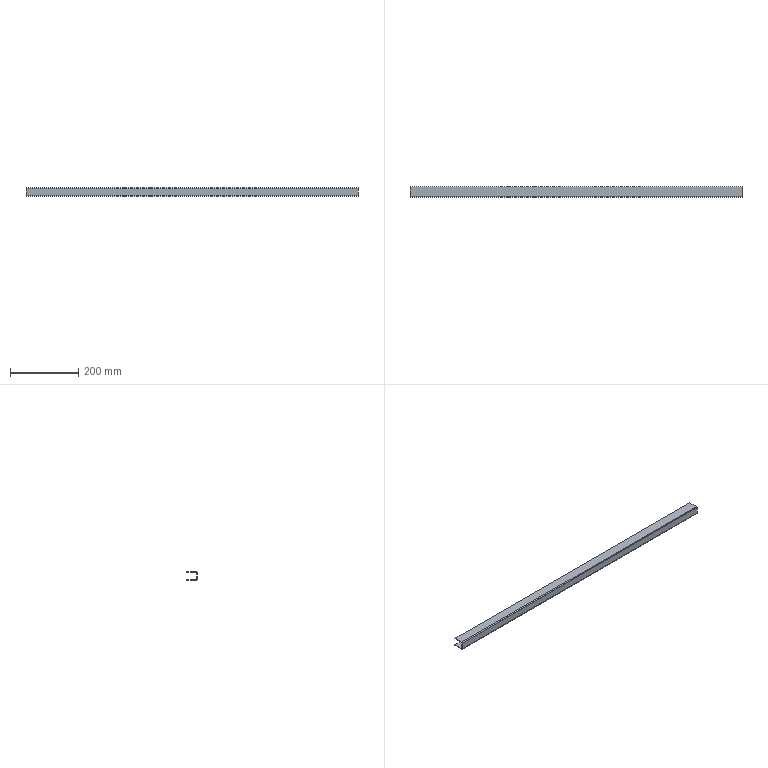Part | NX | features BREP 1 | 1 solid | 14 faces | box 970 x 30 x 25 mm | volume 117124 mm3 | plane 10 | cylinder 4 | commonest cylinder face diameters 2 x2 5 x2
STEP:
#1=CARTESIAN_POINT('',(485.,2.5,11.));
#2=VERTEX_POINT('',#1);
#3=CARTESIAN_POINT('',(485.,1.5,10.));
#4=VERTEX_POINT('',#3);
#5=CARTESIAN_POINT('',(485.,2.5,10.));
#6=DIRECTION('',(1.,0.,0.));
#7=DIRECTION('',(0.,0.,-1.));
#8=AXIS2_PLACEMENT_3D('',#5,#6,#7);
#9=CIRCLE('',#8,1.);
#10=EDGE_CURVE('',#2,#4,#9,.T.);
#11=ORIENTED_EDGE('',*,*,#10,.F.);
#12=CARTESIAN_POINT('',(485.,30.,11.));
#13=VERTEX_POINT('',#12);
#14=CARTESIAN_POINT('',(485.,30.,11.));
#15=DIRECTION('',(0.,-1.,0.));
#16=VECTOR('',#15,1000.);
#17=LINE('',#14,#16);
#18=EDGE_CURVE('',#13,#2,#17,.T.);
#19=ORIENTED_EDGE('',*,*,#18,.F.);
#20=CARTESIAN_POINT('',(485.,30.,12.5));
#21=VERTEX_POINT('',#20);
#22=CARTESIAN_POINT('',(485.,30.,12.5));
#23=DIRECTION('',(0.,0.,-1.));
#24=VECTOR('',#23,1000.);
#25=LINE('',#22,#24);
#26=EDGE_CURVE('',#21,#13,#25,.T.);
#27=ORIENTED_EDGE('',*,*,#26,.F.);
#28=CARTESIAN_POINT('',(485.,2.5,12.5));
#29=VERTEX_POINT('',#28);
#30=CARTESIAN_POINT('',(485.,30.,12.5));
#31=DIRECTION('',(0.,-1.,0.));
#32=VECTOR('',#31,1000.);
#33=LINE('',#30,#32);
#34=EDGE_CURVE('',#21,#29,#33,.T.);
#35=ORIENTED_EDGE('',*,*,#34,.T.);
#36=CARTESIAN_POINT('',(485.,0.,10.));
#37=VERTEX_POINT('',#36);
#38=CARTESIAN_POINT('',(485.,2.5,10.));
#39=DIRECTION('',(1.,0.,0.));
#40=DIRECTION('',(0.,0.,1.));
#41=AXIS2_PLACEMENT_3D('',#38,#39,#40);
#42=CIRCLE('',#41,2.5);
#43=EDGE_CURVE('',#29,#37,#42,.T.);
#44=ORIENTED_EDGE('',*,*,#43,.T.);
#45=CARTESIAN_POINT('',(485.,0.,-10.));
#46=VERTEX_POINT('',#45);
#47=CARTESIAN_POINT('',(485.,0.,12.5));
#48=DIRECTION('',(0.,0.,-1.));
#49=VECTOR('',#48,1000.);
#50=LINE('',#47,#49);
#51=EDGE_CURVE('',#37,#46,#50,.T.);
#52=ORIENTED_EDGE('',*,*,#51,.T.);
#53=CARTESIAN_POINT('',(485.,2.5,-12.5));
#54=VERTEX_POINT('',#53);
#55=CARTESIAN_POINT('',(485.,2.5,-10.));
#56=DIRECTION('',(1.,0.,0.));
#57=DIRECTION('',(0.,0.,1.));
#58=AXIS2_PLACEMENT_3D('',#55,#56,#57);
#59=CIRCLE('',#58,2.5);
#60=EDGE_CURVE('',#46,#54,#59,.T.);
#61=ORIENTED_EDGE('',*,*,#60,.T.);
#62=CARTESIAN_POINT('',(485.,30.,-12.5));
#63=VERTEX_POINT('',#62);
#64=CARTESIAN_POINT('',(485.,0.,-12.5));
#65=DIRECTION('',(0.,1.,0.));
#66=VECTOR('',#65,1000.);
#67=LINE('',#64,#66);
#68=EDGE_CURVE('',#54,#63,#67,.T.);
#69=ORIENTED_EDGE('',*,*,#68,.T.);
#70=CARTESIAN_POINT('',(485.,30.,-11.));
#71=VERTEX_POINT('',#70);
#72=CARTESIAN_POINT('',(485.,30.,-11.));
#73=DIRECTION('',(0.,0.,-1.));
#74=VECTOR('',#73,1000.);
#75=LINE('',#72,#74);
#76=EDGE_CURVE('',#71,#63,#75,.T.);
#77=ORIENTED_EDGE('',*,*,#76,.F.);
#78=CARTESIAN_POINT('',(485.,2.5,-11.));
#79=VERTEX_POINT('',#78);
#80=CARTESIAN_POINT('',(485.,0.,-11.));
#81=DIRECTION('',(0.,1.,0.));
#82=VECTOR('',#81,1000.);
#83=LINE('',#80,#82);
#84=EDGE_CURVE('',#79,#71,#83,.T.);
#85=ORIENTED_EDGE('',*,*,#84,.F.);
#86=CARTESIAN_POINT('',(485.,1.5,-10.));
#87=VERTEX_POINT('',#86);
#88=CARTESIAN_POINT('',(485.,2.5,-10.));
#89=DIRECTION('',(1.,0.,0.));
#90=DIRECTION('',(0.,0.,-1.));
#91=AXIS2_PLACEMENT_3D('',#88,#89,#90);
#92=CIRCLE('',#91,1.);
#93=EDGE_CURVE('',#87,#79,#92,.T.);
#94=ORIENTED_EDGE('',*,*,#93,.F.);
#95=CARTESIAN_POINT('',(485.,1.5,12.5));
#96=DIRECTION('',(0.,0.,-1.));
#97=VECTOR('',#96,1000.);
#98=LINE('',#95,#97);
#99=EDGE_CURVE('',#4,#87,#98,.T.);
#100=ORIENTED_EDGE('',*,*,#99,.F.);
#101=EDGE_LOOP('',(#11,#19,#27,#35,#44,#52,#61,#69,#77,#85,#94,#100));
#102=FACE_BOUND('',#101,.T.);
#103=CARTESIAN_POINT('',(485.,2.5,12.5));
#104=DIRECTION('',(1.,0.,0.));
#105=DIRECTION('',(0.,0.,-1.));
#106=AXIS2_PLACEMENT_3D('',#103,#104,#105);
#107=PLANE('',#106);
#108=ADVANCED_FACE('',(#102),#107,.T.);
#109=CARTESIAN_POINT('',(-485.,2.5,11.));
#110=VERTEX_POINT('',#109);
#111=CARTESIAN_POINT('',(-485.,1.5,10.));
#112=VERTEX_POINT('',#111);
#113=CARTESIAN_POINT('',(-485.,2.5,10.));
#114=DIRECTION('',(1.,0.,0.));
#115=DIRECTION('',(0.,0.,-1.));
#116=AXIS2_PLACEMENT_3D('',#113,#114,#115);
#117=CIRCLE('',#116,1.);
#118=EDGE_CURVE('',#110,#112,#117,.T.);
#119=ORIENTED_EDGE('',*,*,#118,.T.);
#120=CARTESIAN_POINT('',(-485.,1.5,-10.));
#121=VERTEX_POINT('',#120);
#122=CARTESIAN_POINT('',(-485.,1.5,12.5));
#123=DIRECTION('',(0.,0.,-1.));
#124=VECTOR('',#123,1000.);
#125=LINE('',#122,#124);
#126=EDGE_CURVE('',#112,#121,#125,.T.);
#127=ORIENTED_EDGE('',*,*,#126,.T.);
#128=CARTESIAN_POINT('',(-485.,2.5,-11.));
#129=VERTEX_POINT('',#128);
#130=CARTESIAN_POINT('',(-485.,2.5,-10.));
#131=DIRECTION('',(1.,0.,0.));
#132=DIRECTION('',(0.,0.,-1.));
#133=AXIS2_PLACEMENT_3D('',#130,#131,#132);
#134=CIRCLE('',#133,1.);
#135=EDGE_CURVE('',#121,#129,#134,.T.);
#136=ORIENTED_EDGE('',*,*,#135,.T.);
#137=CARTESIAN_POINT('',(-485.,30.,-11.));
#138=VERTEX_POINT('',#137);
#139=CARTESIAN_POINT('',(-485.,0.,-11.));
#140=DIRECTION('',(0.,1.,0.));
#141=VECTOR('',#140,1000.);
#142=LINE('',#139,#141);
#143=EDGE_CURVE('',#129,#138,#142,.T.);
#144=ORIENTED_EDGE('',*,*,#143,.T.);
#145=CARTESIAN_POINT('',(-485.,30.,-12.5));
#146=VERTEX_POINT('',#145);
#147=CARTESIAN_POINT('',(-485.,30.,-11.));
#148=DIRECTION('',(0.,0.,-1.));
#149=VECTOR('',#148,1000.);
#150=LINE('',#147,#149);
#151=EDGE_CURVE('',#138,#146,#150,.T.);
#152=ORIENTED_EDGE('',*,*,#151,.T.);
#153=CARTESIAN_POINT('',(-485.,2.5,-12.5));
#154=VERTEX_POINT('',#153);
#155=CARTESIAN_POINT('',(-485.,0.,-12.5));
#156=DIRECTION('',(0.,1.,0.));
#157=VECTOR('',#156,1000.);
#158=LINE('',#155,#157);
#159=EDGE_CURVE('',#154,#146,#158,.T.);
#160=ORIENTED_EDGE('',*,*,#159,.F.);
#161=CARTESIAN_POINT('',(-485.,0.,-10.));
#162=VERTEX_POINT('',#161);
#163=CARTESIAN_POINT('',(-485.,2.5,-10.));
#164=DIRECTION('',(1.,0.,0.));
#165=DIRECTION('',(0.,0.,1.));
#166=AXIS2_PLACEMENT_3D('',#163,#164,#165);
#167=CIRCLE('',#166,2.5);
#168=EDGE_CURVE('',#162,#154,#167,.T.);
#169=ORIENTED_EDGE('',*,*,#168,.F.);
#170=CARTESIAN_POINT('',(-485.,0.,10.));
#171=VERTEX_POINT('',#170);
#172=CARTESIAN_POINT('',(-485.,0.,12.5));
#173=DIRECTION('',(0.,0.,-1.));
#174=VECTOR('',#173,1000.);
#175=LINE('',#172,#174);
#176=EDGE_CURVE('',#171,#162,#175,.T.);
#177=ORIENTED_EDGE('',*,*,#176,.F.);
#178=CARTESIAN_POINT('',(-485.,2.5,12.5));
#179=VERTEX_POINT('',#178);
#180=CARTESIAN_POINT('',(-485.,2.5,10.));
#181=DIRECTION('',(1.,0.,0.));
#182=DIRECTION('',(0.,0.,1.));
#183=AXIS2_PLACEMENT_3D('',#180,#181,#182);
#184=CIRCLE('',#183,2.5);
#185=EDGE_CURVE('',#179,#171,#184,.T.);
#186=ORIENTED_EDGE('',*,*,#185,.F.);
#187=CARTESIAN_POINT('',(-485.,30.,12.5));
#188=VERTEX_POINT('',#187);
#189=CARTESIAN_POINT('',(-485.,30.,12.5));
#190=DIRECTION('',(0.,-1.,0.));
#191=VECTOR('',#190,1000.);
#192=LINE('',#189,#191);
#193=EDGE_CURVE('',#188,#179,#192,.T.);
#194=ORIENTED_EDGE('',*,*,#193,.F.);
#195=CARTESIAN_POINT('',(-485.,30.,11.));
#196=VERTEX_POINT('',#195);
#197=CARTESIAN_POINT('',(-485.,30.,12.5));
#198=DIRECTION('',(0.,0.,-1.));
#199=VECTOR('',#198,1000.);
#200=LINE('',#197,#199);
#201=EDGE_CURVE('',#188,#196,#200,.T.);
#202=ORIENTED_EDGE('',*,*,#201,.T.);
#203=CARTESIAN_POINT('',(-485.,30.,11.));
#204=DIRECTION('',(0.,-1.,0.));
#205=VECTOR('',#204,1000.);
#206=LINE('',#203,#205);
#207=EDGE_CURVE('',#196,#110,#206,.T.);
#208=ORIENTED_EDGE('',*,*,#207,.T.);
#209=EDGE_LOOP('',(#119,#127,#136,#144,#152,#160,#169,#177,#186,#194,#202,#208));
#210=FACE_BOUND('',#209,.T.);
#211=CARTESIAN_POINT('',(-485.,0.,10.));
#212=DIRECTION('',(-1.,0.,0.));
#213=DIRECTION('',(0.,0.,1.));
#214=AXIS2_PLACEMENT_3D('',#211,#212,#213);
#215=PLANE('',#214);
#216=ADVANCED_FACE('',(#210),#215,.T.);
#217=ORIENTED_EDGE('',*,*,#159,.T.);
#218=CARTESIAN_POINT('',(485.,30.,-12.5));
#219=DIRECTION('',(-1.,0.,0.));
#220=VECTOR('',#219,1000.);
#221=LINE('',#218,#220);
#222=EDGE_CURVE('',#63,#146,#221,.T.);
#223=ORIENTED_EDGE('',*,*,#222,.F.);
#224=ORIENTED_EDGE('',*,*,#68,.F.);
#225=CARTESIAN_POINT('',(485.,2.5,-12.5));
#226=DIRECTION('',(-1.,0.,0.));
#227=VECTOR('',#226,1000.);
#228=LINE('',#225,#227);
#229=EDGE_CURVE('',#54,#154,#228,.T.);
#230=ORIENTED_EDGE('',*,*,#229,.T.);
#231=EDGE_LOOP('',(#217,#223,#224,#230));
#232=FACE_BOUND('',#231,.T.);
#233=CARTESIAN_POINT('',(485.,0.,-12.5));
#234=DIRECTION('',(0.,0.,1.));
#235=DIRECTION('',(0.,-1.,0.));
#236=AXIS2_PLACEMENT_3D('',#233,#234,#235);
#237=PLANE('',#236);
#238=ADVANCED_FACE('',(#232),#237,.F.);
#239=ORIENTED_EDGE('',*,*,#151,.F.);
#240=CARTESIAN_POINT('',(485.,30.,-11.));
#241=DIRECTION('',(-1.,0.,0.));
#242=VECTOR('',#241,1000.);
#243=LINE('',#240,#242);
#244=EDGE_CURVE('',#71,#138,#243,.T.);
#245=ORIENTED_EDGE('',*,*,#244,.F.);
#246=ORIENTED_EDGE('',*,*,#76,.T.);
#247=ORIENTED_EDGE('',*,*,#222,.T.);
#248=EDGE_LOOP('',(#239,#245,#246,#247));
#249=FACE_BOUND('',#248,.T.);
#250=CARTESIAN_POINT('',(485.,30.,-11.));
#251=DIRECTION('',(0.,1.,0.));
#252=DIRECTION('',(0.,0.,1.));
#253=AXIS2_PLACEMENT_3D('',#250,#251,#252);
#254=PLANE('',#253);
#255=ADVANCED_FACE('',(#249),#254,.T.);
#256=ORIENTED_EDGE('',*,*,#143,.F.);
#257=CARTESIAN_POINT('',(485.,2.5,-11.));
#258=DIRECTION('',(-1.,0.,0.));
#259=VECTOR('',#258,1000.);
#260=LINE('',#257,#259);
#261=EDGE_CURVE('',#79,#129,#260,.T.);
#262=ORIENTED_EDGE('',*,*,#261,.F.);
#263=ORIENTED_EDGE('',*,*,#84,.T.);
#264=ORIENTED_EDGE('',*,*,#244,.T.);
#265=EDGE_LOOP('',(#256,#262,#263,#264));
#266=FACE_BOUND('',#265,.T.);
#267=CARTESIAN_POINT('',(485.,0.,-11.));
#268=DIRECTION('',(0.,0.,1.));
#269=DIRECTION('',(0.,-1.,0.));
#270=AXIS2_PLACEMENT_3D('',#267,#268,#269);
#271=PLANE('',#270);
#272=ADVANCED_FACE('',(#266),#271,.T.);
#273=ORIENTED_EDGE('',*,*,#135,.F.);
#274=CARTESIAN_POINT('',(485.,1.5,-10.));
#275=DIRECTION('',(-1.,0.,0.));
#276=VECTOR('',#275,1000.);
#277=LINE('',#274,#276);
#278=EDGE_CURVE('',#87,#121,#277,.T.);
#279=ORIENTED_EDGE('',*,*,#278,.F.);
#280=ORIENTED_EDGE('',*,*,#93,.T.);
#281=ORIENTED_EDGE('',*,*,#261,.T.);
#282=EDGE_LOOP('',(#273,#279,#280,#281));
#283=FACE_BOUND('',#282,.T.);
#284=CARTESIAN_POINT('',(485.,2.5,-10.));
#285=DIRECTION('',(-1.,0.,0.));
#286=DIRECTION('',(0.,0.,1.));
#287=AXIS2_PLACEMENT_3D('',#284,#285,#286);
#288=CYLINDRICAL_SURFACE('',#287,1.);
#289=ADVANCED_FACE('',(#283),#288,.F.);
#290=ORIENTED_EDGE('',*,*,#126,.F.);
#291=CARTESIAN_POINT('',(485.,1.5,10.));
#292=DIRECTION('',(-1.,0.,0.));
#293=VECTOR('',#292,1000.);
#294=LINE('',#291,#293);
#295=EDGE_CURVE('',#4,#112,#294,.T.);
#296=ORIENTED_EDGE('',*,*,#295,.F.);
#297=ORIENTED_EDGE('',*,*,#99,.T.);
#298=ORIENTED_EDGE('',*,*,#278,.T.);
#299=EDGE_LOOP('',(#290,#296,#297,#298));
#300=FACE_BOUND('',#299,.T.);
#301=CARTESIAN_POINT('',(485.,1.5,12.5));
#302=DIRECTION('',(0.,1.,0.));
#303=DIRECTION('',(0.,0.,1.));
#304=AXIS2_PLACEMENT_3D('',#301,#302,#303);
#305=PLANE('',#304);
#306=ADVANCED_FACE('',(#300),#305,.T.);
#307=ORIENTED_EDGE('',*,*,#118,.F.);
#308=CARTESIAN_POINT('',(485.,2.5,11.));
#309=DIRECTION('',(-1.,0.,0.));
#310=VECTOR('',#309,1000.);
#311=LINE('',#308,#310);
#312=EDGE_CURVE('',#2,#110,#311,.T.);
#313=ORIENTED_EDGE('',*,*,#312,.F.);
#314=ORIENTED_EDGE('',*,*,#10,.T.);
#315=ORIENTED_EDGE('',*,*,#295,.T.);
#316=EDGE_LOOP('',(#307,#313,#314,#315));
#317=FACE_BOUND('',#316,.T.);
#318=CARTESIAN_POINT('',(485.,2.5,10.));
#319=DIRECTION('',(-1.,0.,0.));
#320=DIRECTION('',(0.,0.,1.));
#321=AXIS2_PLACEMENT_3D('',#318,#319,#320);
#322=CYLINDRICAL_SURFACE('',#321,1.);
#323=ADVANCED_FACE('',(#317),#322,.F.);
#324=ORIENTED_EDGE('',*,*,#207,.F.);
#325=CARTESIAN_POINT('',(485.,30.,11.));
#326=DIRECTION('',(-1.,0.,0.));
#327=VECTOR('',#326,1000.);
#328=LINE('',#325,#327);
#329=EDGE_CURVE('',#13,#196,#328,.T.);
#330=ORIENTED_EDGE('',*,*,#329,.F.);
#331=ORIENTED_EDGE('',*,*,#18,.T.);
#332=ORIENTED_EDGE('',*,*,#312,.T.);
#333=EDGE_LOOP('',(#324,#330,#331,#332));
#334=FACE_BOUND('',#333,.T.);
#335=CARTESIAN_POINT('',(485.,30.,11.));
#336=DIRECTION('',(0.,0.,-1.));
#337=DIRECTION('',(0.,1.,0.));
#338=AXIS2_PLACEMENT_3D('',#335,#336,#337);
#339=PLANE('',#338);
#340=ADVANCED_FACE('',(#334),#339,.T.);
#341=ORIENTED_EDGE('',*,*,#201,.F.);
#342=CARTESIAN_POINT('',(485.,30.,12.5));
#343=DIRECTION('',(-1.,0.,0.));
#344=VECTOR('',#343,1000.);
#345=LINE('',#342,#344);
#346=EDGE_CURVE('',#21,#188,#345,.T.);
#347=ORIENTED_EDGE('',*,*,#346,.F.);
#348=ORIENTED_EDGE('',*,*,#26,.T.);
#349=ORIENTED_EDGE('',*,*,#329,.T.);
#350=EDGE_LOOP('',(#341,#347,#348,#349));
#351=FACE_BOUND('',#350,.T.);
#352=CARTESIAN_POINT('',(485.,30.,12.5));
#353=DIRECTION('',(0.,1.,0.));
#354=DIRECTION('',(0.,0.,1.));
#355=AXIS2_PLACEMENT_3D('',#352,#353,#354);
#356=PLANE('',#355);
#357=ADVANCED_FACE('',(#351),#356,.T.);
#358=ORIENTED_EDGE('',*,*,#193,.T.);
#359=CARTESIAN_POINT('',(485.,2.5,12.5));
#360=DIRECTION('',(-1.,0.,0.));
#361=VECTOR('',#360,1000.);
#362=LINE('',#359,#361);
#363=EDGE_CURVE('',#29,#179,#362,.T.);
#364=ORIENTED_EDGE('',*,*,#363,.F.);
#365=ORIENTED_EDGE('',*,*,#34,.F.);
#366=ORIENTED_EDGE('',*,*,#346,.T.);
#367=EDGE_LOOP('',(#358,#364,#365,#366));
#368=FACE_BOUND('',#367,.T.);
#369=CARTESIAN_POINT('',(485.,30.,12.5));
#370=DIRECTION('',(0.,0.,-1.));
#371=DIRECTION('',(0.,1.,0.));
#372=AXIS2_PLACEMENT_3D('',#369,#370,#371);
#373=PLANE('',#372);
#374=ADVANCED_FACE('',(#368),#373,.F.);
#375=ORIENTED_EDGE('',*,*,#185,.T.);
#376=CARTESIAN_POINT('',(485.,0.,10.));
#377=DIRECTION('',(-1.,0.,0.));
#378=VECTOR('',#377,1000.);
#379=LINE('',#376,#378);
#380=EDGE_CURVE('',#37,#171,#379,.T.);
#381=ORIENTED_EDGE('',*,*,#380,.F.);
#382=ORIENTED_EDGE('',*,*,#43,.F.);
#383=ORIENTED_EDGE('',*,*,#363,.T.);
#384=EDGE_LOOP('',(#375,#381,#382,#383));
#385=FACE_BOUND('',#384,.T.);
#386=CARTESIAN_POINT('',(485.,2.5,10.));
#387=DIRECTION('',(-1.,0.,0.));
#388=DIRECTION('',(0.,0.,1.));
#389=AXIS2_PLACEMENT_3D('',#386,#387,#388);
#390=CYLINDRICAL_SURFACE('',#389,2.5);
#391=ADVANCED_FACE('',(#385),#390,.T.);
#392=ORIENTED_EDGE('',*,*,#176,.T.);
#393=CARTESIAN_POINT('',(485.,0.,-10.));
#394=DIRECTION('',(-1.,0.,0.));
#395=VECTOR('',#394,1000.);
#396=LINE('',#393,#395);
#397=EDGE_CURVE('',#46,#162,#396,.T.);
#398=ORIENTED_EDGE('',*,*,#397,.F.);
#399=ORIENTED_EDGE('',*,*,#51,.F.);
#400=ORIENTED_EDGE('',*,*,#380,.T.);
#401=EDGE_LOOP('',(#392,#398,#399,#400));
#402=FACE_BOUND('',#401,.T.);
#403=CARTESIAN_POINT('',(485.,0.,12.5));
#404=DIRECTION('',(0.,1.,0.));
#405=DIRECTION('',(0.,0.,1.));
#406=AXIS2_PLACEMENT_3D('',#403,#404,#405);
#407=PLANE('',#406);
#408=ADVANCED_FACE('',(#402),#407,.F.);
#409=ORIENTED_EDGE('',*,*,#168,.T.);
#410=ORIENTED_EDGE('',*,*,#229,.F.);
#411=ORIENTED_EDGE('',*,*,#60,.F.);
#412=ORIENTED_EDGE('',*,*,#397,.T.);
#413=EDGE_LOOP('',(#409,#410,#411,#412));
#414=FACE_BOUND('',#413,.T.);
#415=CARTESIAN_POINT('',(485.,2.5,-10.));
#416=DIRECTION('',(-1.,0.,0.));
#417=DIRECTION('',(0.,0.,1.));
#418=AXIS2_PLACEMENT_3D('',#415,#416,#417);
#419=CYLINDRICAL_SURFACE('',#418,2.5);
#420=ADVANCED_FACE('',(#414),#419,.T.);
#421=CLOSED_SHELL('',(#108,#216,#238,#255,#272,#289,#306,#323,#340,#357,#374,#391,#408,#420));
#422=MANIFOLD_SOLID_BREP('',#421);
#423=(LENGTH_UNIT()NAMED_UNIT(*)SI_UNIT(.MILLI.,.METRE.));
#424=UNCERTAINTY_MEASURE_WITH_UNIT(LENGTH_MEASURE(0.00001),#423,'','');
#425=(NAMED_UNIT(*)PLANE_ANGLE_UNIT()SI_UNIT($,.RADIAN.));
#426=(NAMED_UNIT(*)SI_UNIT($,.STERADIAN.)SOLID_ANGLE_UNIT());
#427=(GEOMETRIC_REPRESENTATION_CONTEXT(3)GLOBAL_UNCERTAINTY_ASSIGNED_CONTEXT((#424))GLOBAL_UNIT_ASSIGNED_CONTEXT((#423,#425,#426))REPRESENTATION_CONTEXT('',''));
#428=ADVANCED_BREP_SHAPE_REPRESENTATION('',(#422),#427);